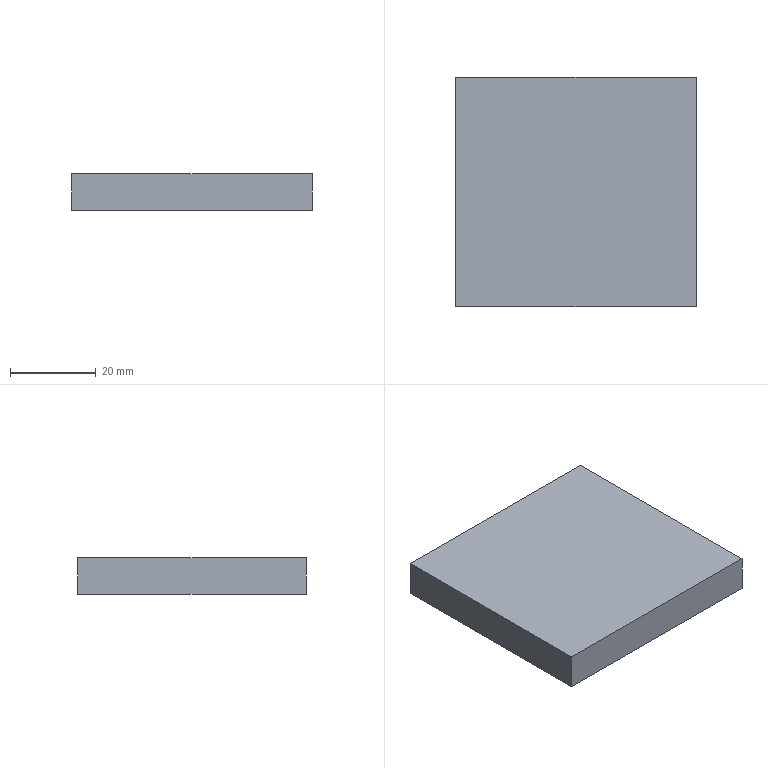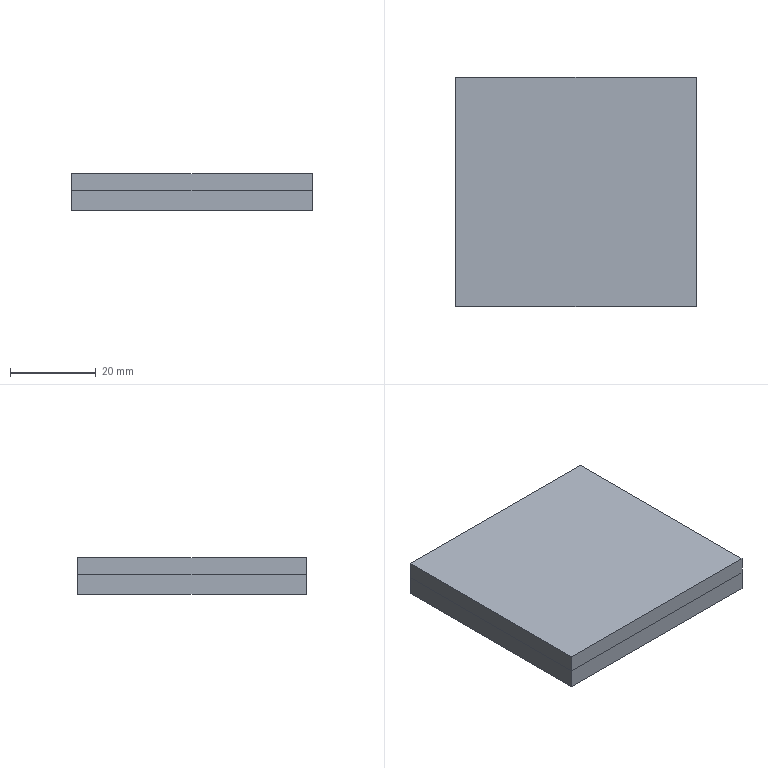CAM job | NX | 3-axis milling, drilling | part box 56 x 53.3 x 8.5 mm | stock box 56 x 53.3 x 8.5 mm
Tools:
number,name,description,diameter,corner_radius,flute_length,length,flutes
19,D80,Milling Tool-5 Parameters,80.0,0.0,50.0,75.0,2
1,D6A45,Milling Tool-5 Parameters,6.0,0.0,50.0,75.0,2
16,2.0ZT,Drilling Tool,2.0,0.0,35.0,50.0,2
17,2.4ZT,Drilling Tool,2.4,0.0,35.0,50.0,2
15,D10,Milling Tool-5 Parameters,10.0,0.0,50.0,75.0,2
11,D4,Milling Tool-5 Parameters,4.0,0.0,50.0,75.0,2
18,D2,Milling Tool-5 Parameters,2.0,0.0,50.0,75.0,2
12,D6,Milling Tool-5 Parameters,6.0,0.0,50.0,75.0,2
20,D1.5,Milling Tool-5 Parameters,1.5,0.0,50.0,75.0,2
Operations:
program,operation,operation_type,tool,method,geometry_group,spindle_rpm,surface_speed,feed_per_tooth,feed_cut,feed_plunge,cut_length_mm,path_length_mm,cut_time_min,machine_time_min
1,FLOOR_WALL_COPY,VolumeBased25DMillingOperation,D80,METHOD,A,6500.0,1633.0,0.1154,1500.0,100.0,152.0,206.0,0.1013,0.1067
1,DRILLING_COPY_1,Operation,D6A45,METHOD,A,5000.0,94.0,0.035,350.0,0.0,16.0,157.872,0.0457,0.0599
1,DRILLING_COPY_1_COPY,Operation,2.0ZT,METHOD,A,2000.0,12.0,0.0375,150.0,0.0,12.202,102.388,0.0813,0.0904
1,DRILLING_COPY_1_COPY_COPY,Operation,2.4ZT,METHOD,A,2000.0,12.0,0.0375,150.0,0.0,17.442,135.739,0.1163,0.1281
1,ADAPTIVE_MILLING,CavityMilling,D10,METHOD,A,9500.0,298.0,0.1579,3000.0,1000.0,2334.051,2395.051,0.78,0.7861
1,ZLEVEL_PROFILE,ZLevelMilling,D4,METHOD,A,9500.0,119.0,0.0868,1650.0,1000.0,447.571,1257.897,0.3015,0.3825
1,HOLE_MILLING,CylinderMilling,D2,METHOD,A,9500.0,59.0,0.0658,1250.0,100.0,269.607,430.743,0.2157,0.2318
1,ZLEVEL_PROFILE_COPY,ZLevelMilling,D2,METHOD,A,9500.0,59.0,0.0632,1200.0,1000.0,253.675,733.401,0.22,0.268
1,PLANAR_MILL_COPY_COPY_COPY_COPY_COPY_COPY_1_COPY_1,PlanarMilling,D6A45,METHOD,A,9500.0,179.0,0.0658,1250.0,100.0,203.294,573.06,0.1626,0.1996
1,刀补11,ZLevelMilling,D4,METHOD,A,9500.0,298.0,0.0632,1200.0,1000.0,168.255,233.255,0.1406,0.1471
2,FLOOR_WALL_COPY_COPY,VolumeBased25DMillingOperation,D80,METHOD,B,6500.0,1633.0,0.1154,1500.0,100.0,426.0,857.001,0.284,0.3271
2,刀补11_COPY_1_COPY,ZLevelMilling,D6,METHOD,B,9500.0,179.0,0.1053,2000.0,1000.0,3320.015,3380.015,1.676,1.682
2,CAVITY_MILL,CavityMilling,D6,METHOD,B,9500.0,179.0,0.1316,2500.0,800.0,2505.343,2750.513,1.113,1.141
2,CAVITY_MILL_COPY,CavityMilling,D4,METHOD,B,9500.0,119.0,0.0632,1200.0,800.0,1153.827,3216.738,1.156,1.378
2,FLOOR_WALL,VolumeBased25DMillingOperation,D4,METHOD,B,9500.0,119.0,0.0579,1100.0,100.0,1422.153,1762.56,1.293,1.327
2,ZLEVEL_PROFILE_COPY_COPY,ZLevelMilling,D2,METHOD,B,9500.0,59.0,0.0579,1100.0,1000.0,552.458,1886.611,0.5077,0.6411
2,PLANAR_MILL_COPY_COPY_COPY_COPY_COPY_COPY_1_COPY_1_COPY,PlanarMilling,D6A45,METHOD,B,9500.0,179.0,0.0658,1250.0,100.0,60.59,339.486,0.0485,0.0764
2,PLANAR_MILL_COPY_COPY_COPY_COPY_COPY_COPY_1_COPY_1_COPY_COPY,PlanarMilling,D6A45,METHOD,B,9500.0,179.0,0.0658,1250.0,100.0,327.899,677.615,0.2623,0.2973
2,HOLE_MILLING_1,CylinderMilling,D1.5,METHOD,B,9500.0,44.0,0.0447,850.0,100.0,63.694,209.375,0.0749,0.0895
2,HOLE_MILLING_1_COPY,CylinderMilling,D1.5,METHOD,B,9500.0,44.0,0.0447,850.0,100.0,291.339,455.075,0.3428,0.3591
2,刀补11_COPY_1,ZLevelMilling,D4,METHOD,B,9500.0,298.0,0.0632,1200.0,1000.0,503.665,568.198,0.4201,0.4265
3,CAVITY_MILL_COPY_1,CavityMilling,D6,METHOD,C,9500.0,179.0,0.1316,2500.0,800.0,2773.671,2921.756,1.3,1.321
3,CAVITY_MILL_COPY_COPY,CavityMilling,D4,METHOD,C,9500.0,119.0,0.0632,1200.0,800.0,924.783,2039.341,0.9115,1.043
3,ZLEVEL_PROFILE_COPY_COPY_COPY,ZLevelMilling,D2,METHOD,C,9500.0,59.0,0.0579,1100.0,1000.0,253.212,712.833,0.2349,0.2809
3,FLOOR_WALL_COPY_1,VolumeBased25DMillingOperation,D4,METHOD,C,9500.0,119.0,0.0579,1100.0,100.0,684.676,745.576,0.6224,0.6285
3,刀补11_COPY,ZLevelMilling,D2,METHOD,C,9500.0,298.0,0.0632,1200.0,1000.0,148.488,213.488,0.124,0.1305